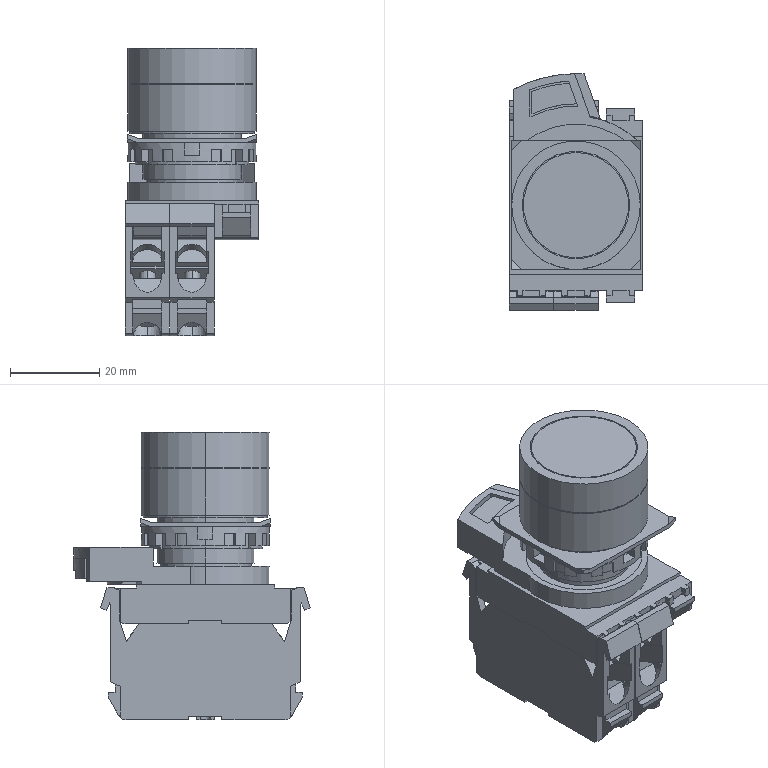Part | STEP file | A22NL_BGM_TGA_G100_GC | 6 solids | 703 faces | box 30 x 53 x 64.4 mm | volume 41405 mm3 | plane 563 | cylinder 140 | commonest cylinder face diameters 6.5 x12 4 x10 25.4 x10 28.8 x9 3.5 x8 5.8 x8